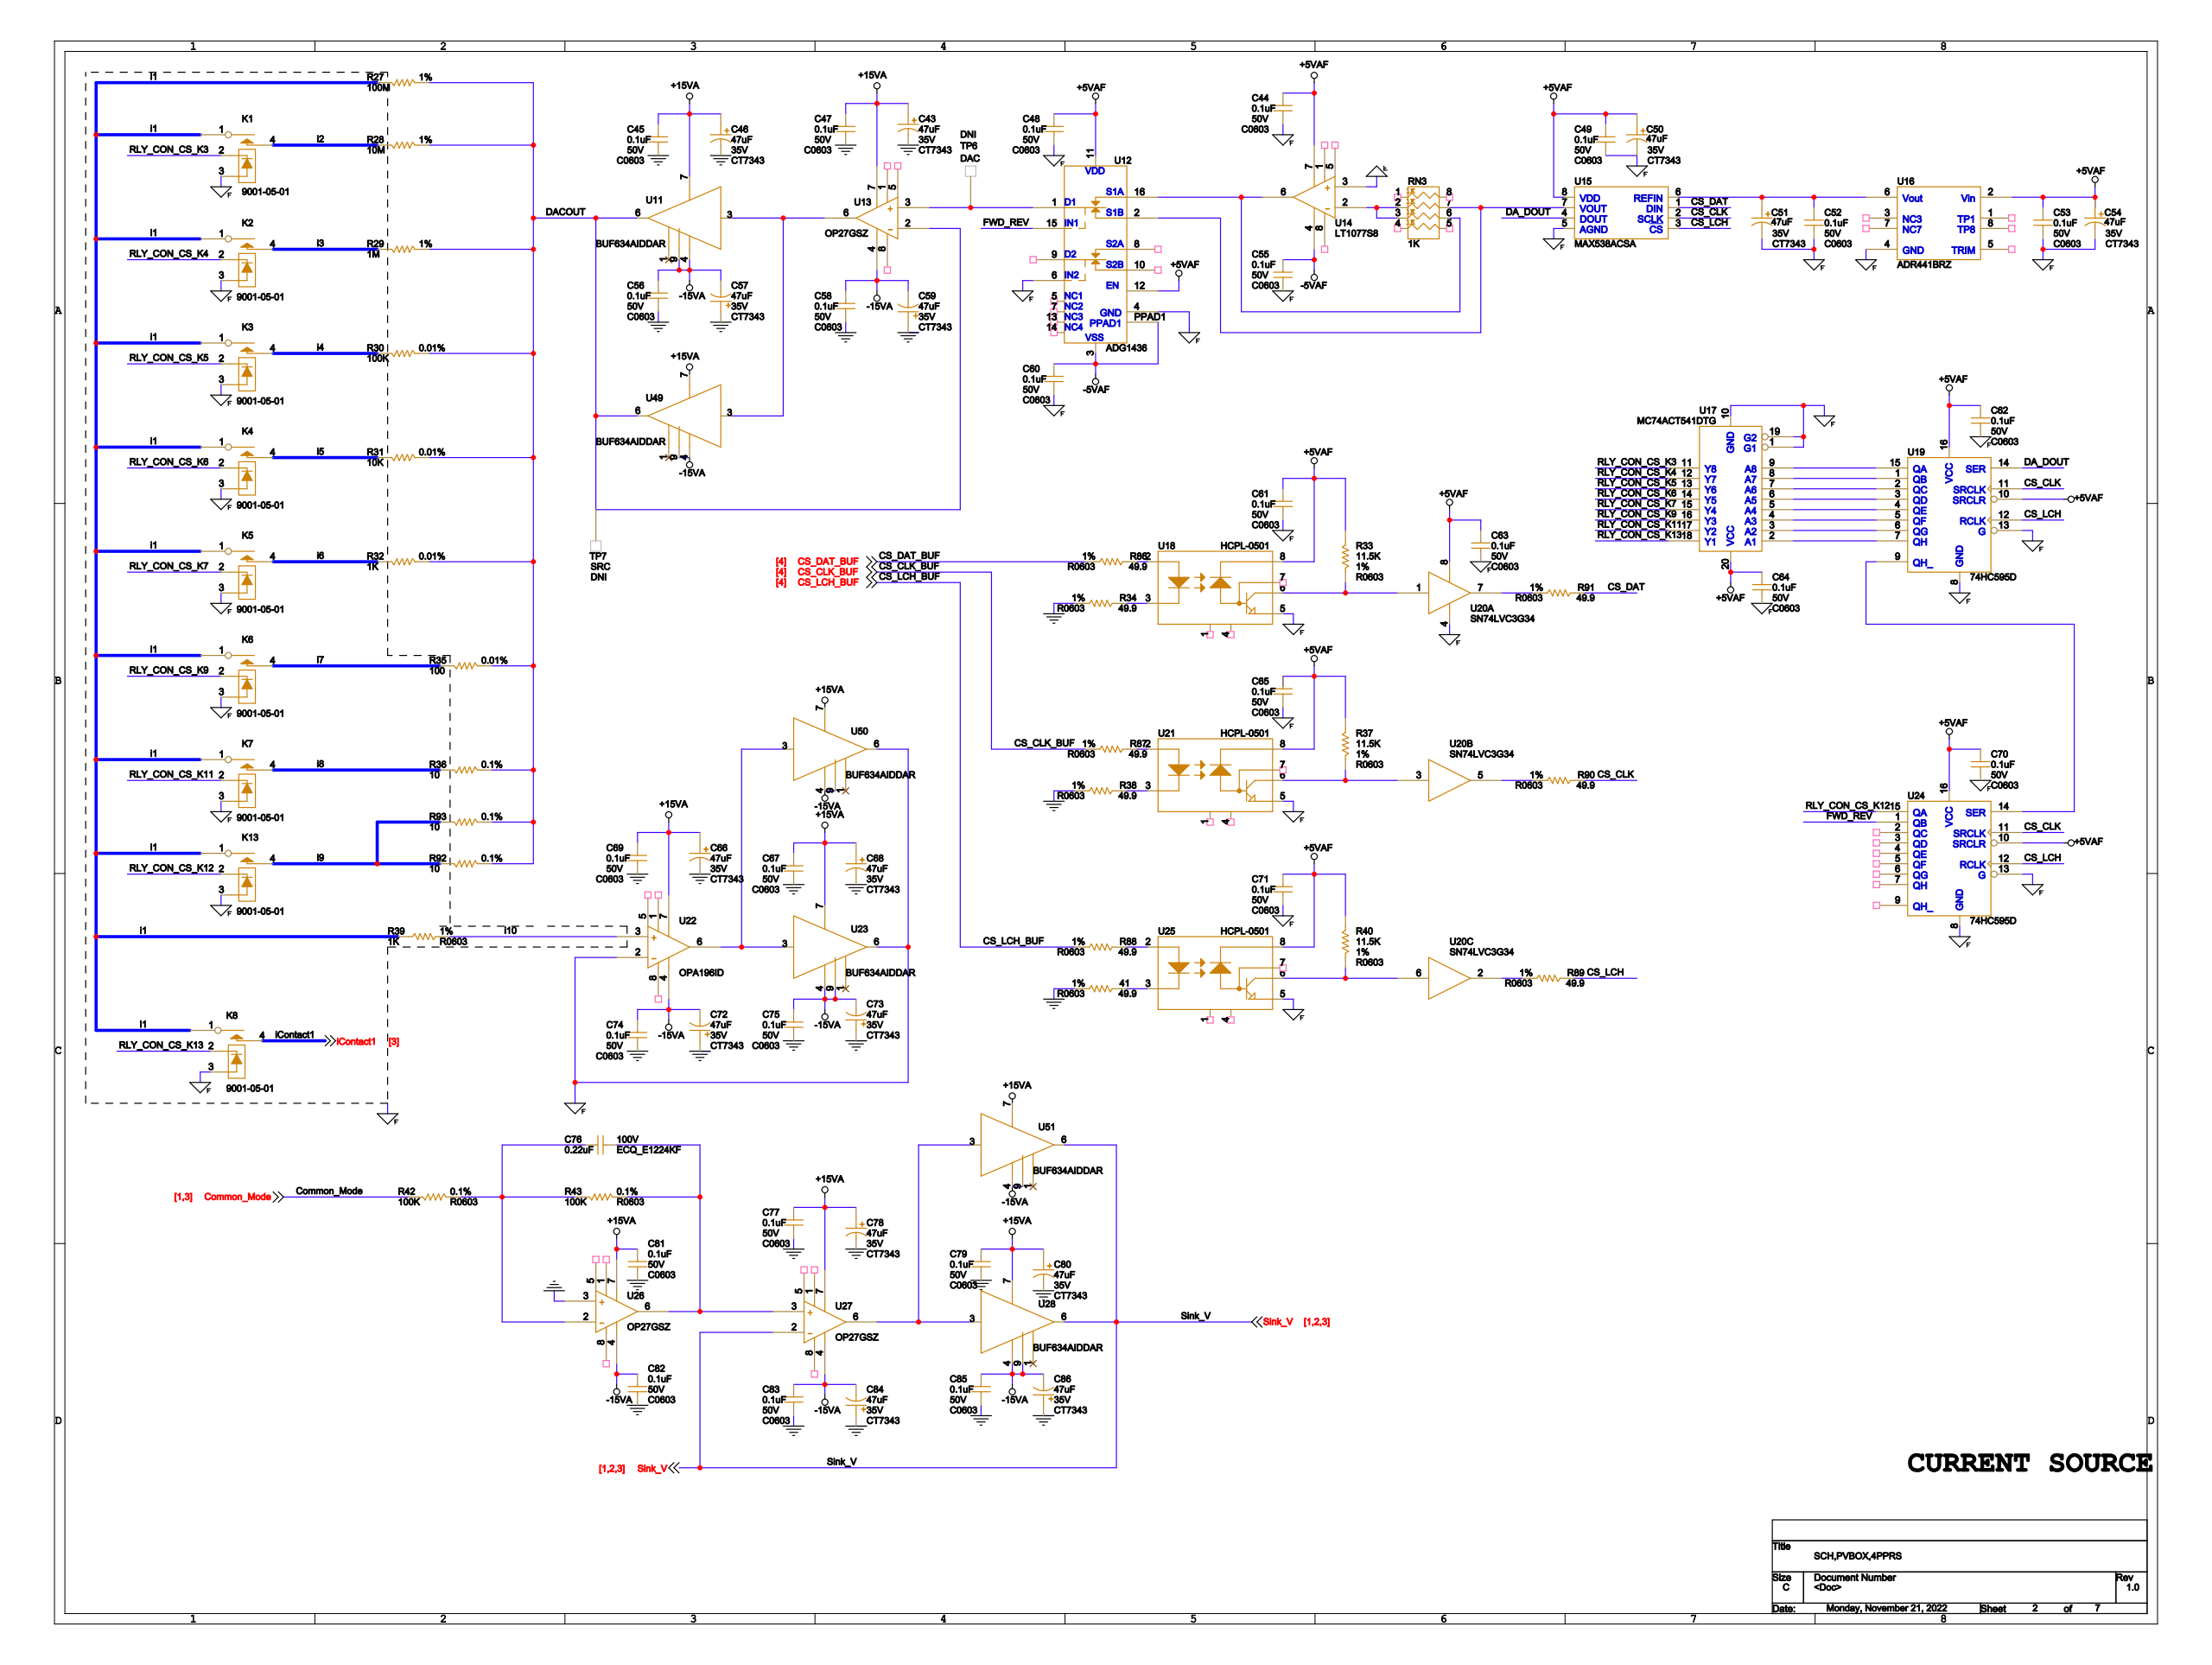Circuit board | Cadence Allegro | 405 parts | 254 nets | one sheet of the schematic
Parts on this sheet (reference | value | footprint):
C43 | CT7343
C44 | C0603
C45 | C0603
C46 | CT7343
C47 | C0603
C48 | C0603
C49 | C0603
C52 | C0603
C53 | C0603
C55 | C0603
C56 | C0603
C57 | CT7343
C58 | C0603
C59 | CT7343
C60 | C0603
C61 | C0603
C62 | C0603
C63 | C0603
C64 | C0603
C65 | C0603
C66 | CT7343
C67 | C0603
C68 | CT7343
C69 | C0603
C70 | C0603
C71 | C0603
C72 | CT7343
C73 | CT7343
C74 | C0603
C75 | C0603
C76 | ECQ_E1224KF
C77 | C0603
C78 | CT7343
C79 | C0603
C80 | CT7343
C81 | C0603
C82 | C0603
C83 | C0603
C84 | CT7343
C85 | C0603
C86 | CT7343
K1 | COTO_9001_5_1
K2 | COTO_9001_5_1
K3 | COTO_9001_5_1
K4 | COTO_9001_5_1
K5 | COTO_9001_5_1
K6 | COTO_9001_5_1
K7 | COTO_9001_5_1
K8 | COTO_9001_5_1
K13 | COTO_9001_5_1
R27 | SM10203
R28 | SM10203
R29 | SM10203
R30 | RD_2_7M87X2M91X8M53_3M81
R31 | RD_2_7M87X2M91X8M53_3M81
R32 | RD_2_7M87X2M91X8M53_3M81
R33 | R0603
R34 | R0603
R35 | RD_2_7M87X2M91X8M53_3M81
R36 | RD_2_7M87X2M91X8M53_3M81
R37 | R0603
R38 | R0603
R39 | R0603
R40 | R0603
R42 | R0603
R43 | R0603
R86 | R0603
R87 | R0603
R88 | R0603
R89 | R0603
R90 | R0603
R91 | R0603
R92 | RD_2_7M87X2M91X8M53_3M81
R93 | RD_2_7M87X2M91X8M53_3M81
RN3 | ACASA
TP6 | TP_0M8X1M15
TP7 | TP_0M8X1M15
U11 | TO220_5_10M67X4M83X16M11_1M7_B
U12 | QFN_17_4MX4MX1M_0M65
U13 | SOIC_8_4MX5MX1M75_1M27
U14 | SOIC_8_4MX5MX1M75_1M27
U15 | SOIC_8_4MX5MX1M75_1M27
U16 | SOIC_8_4MX5MX1M75_1M27
U17 | SOPTS_20_4M5X6M6X1M2_0M65
U18 | SOIC_8_4MX5MX1M75_1M27
U19 | SOIC_16_4MX10MX1M75_1M27
U21 | SOIC_8_4MX5MX1M75_1M27
U22 | SOIC_8_4MX5MX1M75_1M27
U23 | TO220_5_10M67X4M83X16M11_1M7_B
U24 | SOIC_16_4MX10MX1M75_1M27
U25 | SOIC_8_4MX5MX1M75_1M27
U26 | SOIC_8_4MX5MX1M75_1M27
U27 | SOIC_8_4MX5MX1M75_1M27
U28 | TO220_5_10M67X4M83X16M11_1M7_B
U49 | TO220_5_10M67X4M83X16M11_1M7_B
U50 | TO220_5_10M67X4M83X16M11_1M7_B
U51 | TO220_5_10M67X4M83X16M11_1M7_B
Nets of these parts (net: part-pin ...):
N17248519: U25-3
GND: C43-2 C45-2 C46-2 C47-2 C56-2 C57-1 C58-2 C59-1 C66-2 C67-2 C68-2 C69-2 C72-1 C73-1 C74-2 C75-2 C77-2 C78-2 C79-2 C80-2 C81-2 C82-2 C83-2 C84-1 C85-2 C86-1 R34-2 R38-2 U26-3
N17248499: R34-1 U18-3
N17248509: R38-1 U21-3
N19806065: R86-1 U18-2
CS_DAT_BUF: R86-2
N19806082: R87-1 U21-2
CS_CLK_BUF: R87-2
N19806120: R88-1 U25-2
CS_LCH_BUF: R88-2
CS_LCH: R89-1 U15-3 U19-12 U24-12
N17248678: R89-2
CS_CLK: R90-1 U15-2 U19-11 U24-11
N17248675: R90-2
CS_DAT: R91-1 U15-1
N17248672: R91-2
+5VAF: C44-1 C48-1 C49-1 C53-1 C61-1 C62-1 C63-1 C64-1 C65-1 C70-1 C71-1 R33-1 R37-1 R40-1 U12-11 U12-12 U14-7 U15-8 U16-2 U17-20 U18-8 U19-10 U19-16 U21-8 U24-10 U24-16 U25-8
GNDF: C44-2 C48-2 C49-2 C52-2 C53-2 C55-2 C60-2 C61-2 C62-2 C63-2 C64-2 C65-2 C70-2 C71-2 K1-3 K2-3 K3-3 K4-3 K5-3 K6-3 K7-3 K8-3 K13-3 U12-4 U12-6 U14-3 U15-5 U16-4 U17-1 U17-10 U17-19 U18-5 U19-8 U19-13 U21-5 U22-2 U23-6 U24-8 U24-13 U25-5 U50-6
+15VA: C43-1 C45-1 C46-1 C47-1 C66-1 C67-1 C68-1 C69-1 C77-1 C78-1 C79-1 C80-1 C81-1 U11-7 U13-7 U22-7 U23-7 U26-7 U27-7 U28-7 U49-7 U50-7 U51-7
-5VAF: C55-1 C60-1 U12-3 U12-PPAD1 U14-4
-15VA: C56-1 C57-2 C58-1 C59-2 C72-2 C73-2 C74-1 C75-1 C82-1 C83-1 C84-2 C85-1 C86-2 U11-4 U11-9 U13-4 U22-4 U23-4 U23-9 U26-4 U27-4 U28-4 U28-9 U49-4 U49-9 U50-4 U50-9 U51-4 U51-9
N17245734: C52-1 U15-6 U16-6
N19744759: C76-1 R42-1 R43-2 U26-2
N19744760: C76-2 R43-1 U26-6 U27-3
ICONTACT1: K8-4
RLY_CON_CS_K3: K1-2 U17-11
I1: K1-1 K2-1 K3-1 K4-1 K5-1 K6-1 K7-1 K8-1 K13-1 R27-2 R39-1
I2: K1-4 R28-2
RLY_CON_CS_K12: K13-2 U24-15
I9: K13-4 R92-2 R93-2
RLY_CON_CS_K4: K2-2 U17-12
I3: K2-4 R29-2
RLY_CON_CS_K5: K3-2 U17-13
I4: K3-4 R30-2
RLY_CON_CS_K6: K4-2 U17-14
I5: K4-4 R31-2
RLY_CON_CS_K7: K5-2 U17-15
I6: K5-4 R32-2
RLY_CON_CS_K9: K6-2 U17-16
I7: K6-4 R35-2
RLY_CON_CS_K11: K7-2 U17-17
I8: K7-4 R36-2
RLY_CON_CS_K13: K8-2 U17-18
SINK_V: U27-2 U28-6 U51-6
I10: R39-2 U22-3
COMMON_MODE: R42-2
N17248497: R33-2 U18-6
N17248507: R37-2 U21-6
N17248517: R40-2 U25-6
DACOUT: R27-1 R28-1 R29-1 R30-1 R31-1 R32-1 R35-1 R36-1 R92-1 R93-1 TP7-1 U11-6 U13-2 U49-6
N17245843: RN3-2 RN3-3 U14-2
N17245902: RN3-6 U12-16 U14-6
N17245446: RN3-7 U12-2 U15-7
N17832210: TP6-1 U12-1 U13-3
N19744717: U11-3 U13-6 U49-3
N19744677: U22-6 U23-3 U50-3
N19744764: U27-6 U28-3 U51-3
FWD_REV: U12-15 U24-1
DA_DOUT: U15-4 U19-14
N19744870: U17-2 U19-7
N19744869: U17-3 U19-6
N19744868: U17-4 U19-5
N19744867: U17-5 U19-4
N19744866: U17-6 U19-3
N19744865: U17-7 U19-2
N19744864: U17-8 U19-1
N17288551: U17-9 U19-15
N17280955: U19-9 U24-14